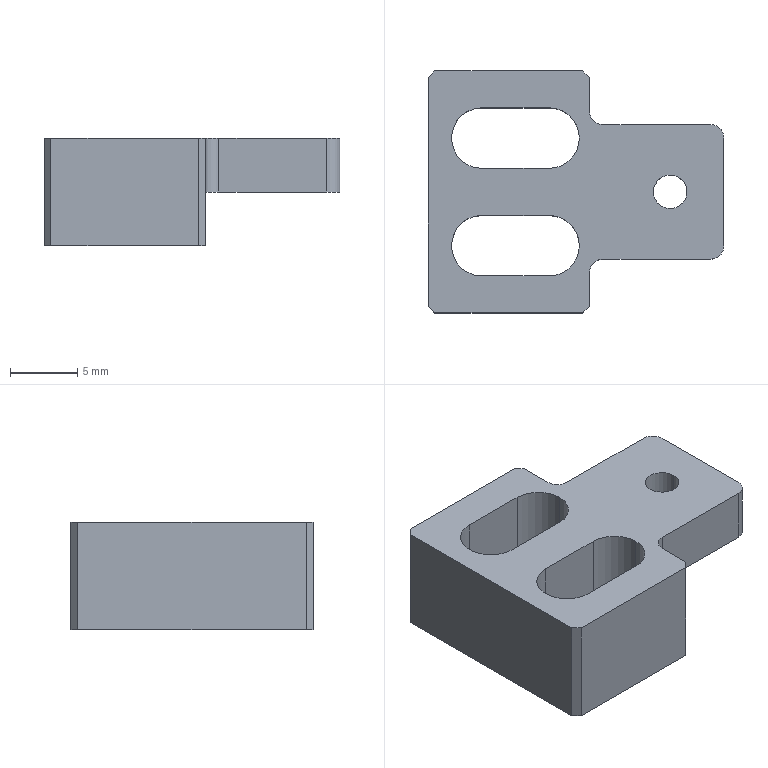Part | STEP file | PN_0030 Mount electronic clip fiber mounting seat A | 1 solid | 30 faces | box 22 x 18 x 8 mm | volume 1490 mm3 | plane 18 | cylinder 12 | commonest cylinder face diameters 4.5 x6 2 x4 2.5 x2